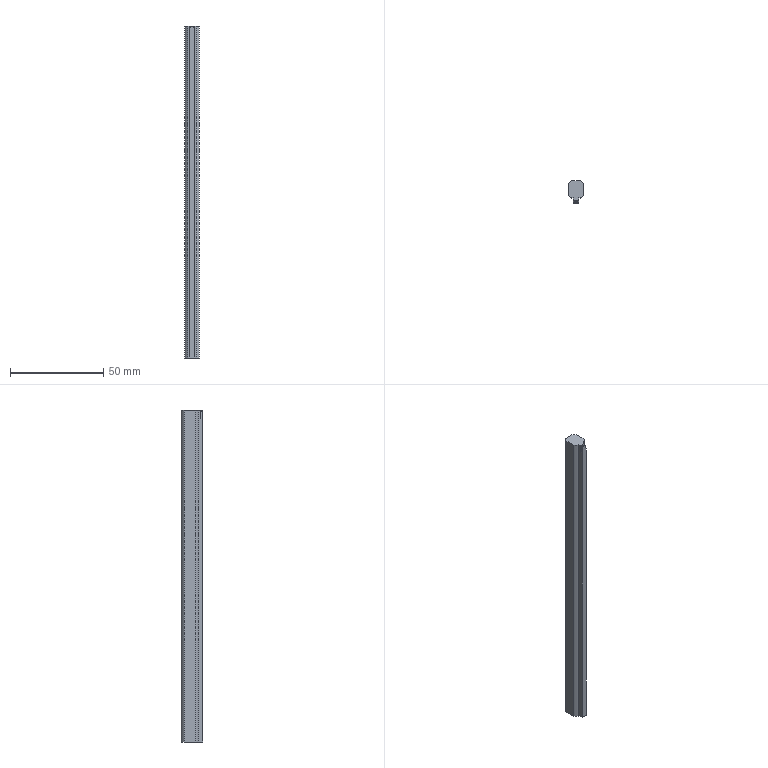Part | STEP file | top shaft | 1 solid | 25 faces | box 8 x 11.5 x 178 mm | volume 13034 mm3 | plane 15 | cylinder 8 | cone 2 | commonest cylinder face diameters 10 x4 0.4 x2 5 x2